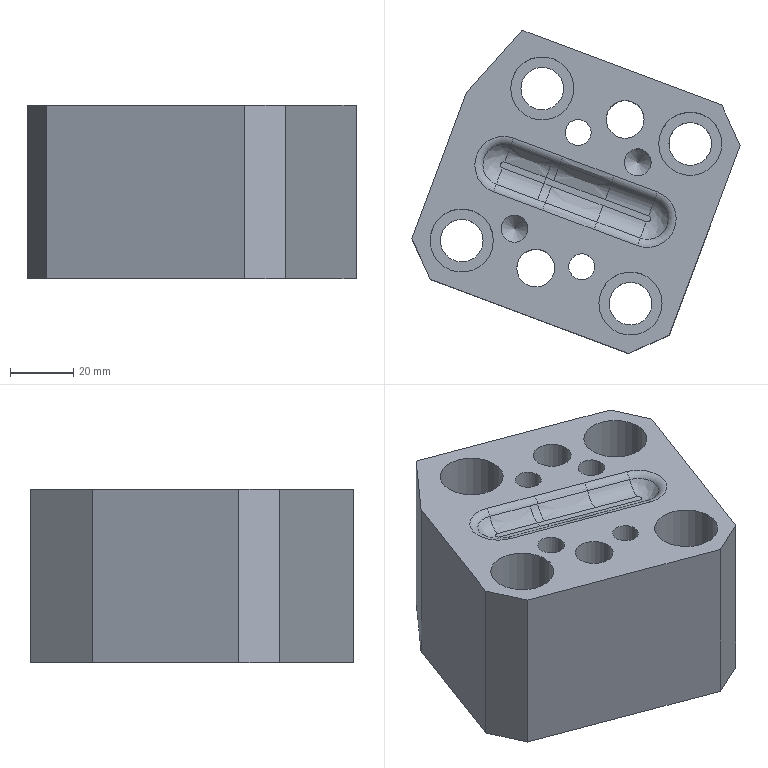Part | NX | features 23 2 | 1 solid | 54 faces | box 103.904 x 102.304 x 55 mm | volume 310584 mm3 | cylinder 24 | plane 18 | spline 8 | torus 2 | cone 2 | commonest cylinder face diameters 6 x4 13 x4 13.5 x4 20 x4 8.2 x2 8.5 x2